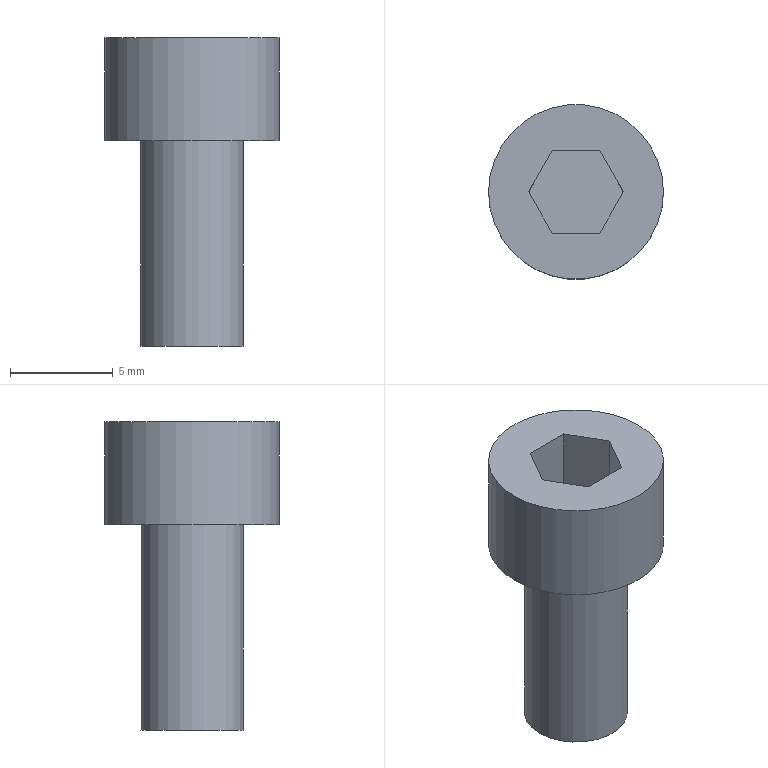Part | STEP file | lll_id514_x_t | 1 solid | 12 faces | box 8.5 x 8.5 x 15 mm | volume 434.348 mm3 | plane 10 | cylinder 2 | commonest cylinder face diameters 5 x1 8.5 x1
STEP:
#1=CARTESIAN_POINT('',(-8.75,0.,127.));
#2=VERTEX_POINT('',#1);
#3=CARTESIAN_POINT('',(-13.,0.,127.));
#4=DIRECTION('',(0.,0.,1.));
#5=DIRECTION('',(1.,0.,0.));
#6=AXIS2_PLACEMENT_3D('',#3,#4,#5);
#7=CIRCLE('',#6,4.25);
#8=EDGE_CURVE('',#2,#2,#7,.T.);
#9=ORIENTED_EDGE('',*,*,#8,.T.);
#10=EDGE_LOOP('',(#9));
#11=FACE_BOUND('',#10,.T.);
#12=CARTESIAN_POINT('',(-14.155,2.,127.));
#13=VERTEX_POINT('',#12);
#14=CARTESIAN_POINT('',(-11.845,2.,127.));
#15=VERTEX_POINT('',#14);
#16=CARTESIAN_POINT('',(-14.155,2.,127.));
#17=DIRECTION('',(1.,0.,0.));
#18=VECTOR('',#17,1.);
#19=LINE('',#16,#18);
#20=EDGE_CURVE('',#13,#15,#19,.T.);
#21=ORIENTED_EDGE('',*,*,#20,.T.);
#22=CARTESIAN_POINT('',(-10.691,0.,127.));
#23=VERTEX_POINT('',#22);
#24=CARTESIAN_POINT('',(-11.845,2.,127.));
#25=DIRECTION('',(0.5,-0.866,0.));
#26=VECTOR('',#25,1.);
#27=LINE('',#24,#26);
#28=EDGE_CURVE('',#15,#23,#27,.T.);
#29=ORIENTED_EDGE('',*,*,#28,.T.);
#30=CARTESIAN_POINT('',(-11.845,-2.,127.));
#31=VERTEX_POINT('',#30);
#32=CARTESIAN_POINT('',(-10.691,0.,127.));
#33=DIRECTION('',(-0.5,-0.866,0.));
#34=VECTOR('',#33,1.);
#35=LINE('',#32,#34);
#36=EDGE_CURVE('',#23,#31,#35,.T.);
#37=ORIENTED_EDGE('',*,*,#36,.T.);
#38=CARTESIAN_POINT('',(-14.155,-2.,127.));
#39=VERTEX_POINT('',#38);
#40=CARTESIAN_POINT('',(-11.845,-2.,127.));
#41=DIRECTION('',(-1.,0.,0.));
#42=VECTOR('',#41,1.);
#43=LINE('',#40,#42);
#44=EDGE_CURVE('',#31,#39,#43,.T.);
#45=ORIENTED_EDGE('',*,*,#44,.T.);
#46=CARTESIAN_POINT('',(-15.309,0.,127.));
#47=VERTEX_POINT('',#46);
#48=CARTESIAN_POINT('',(-14.155,-2.,127.));
#49=DIRECTION('',(-0.5,0.866,0.));
#50=VECTOR('',#49,1.);
#51=LINE('',#48,#50);
#52=EDGE_CURVE('',#39,#47,#51,.T.);
#53=ORIENTED_EDGE('',*,*,#52,.T.);
#54=CARTESIAN_POINT('',(-15.309,0.,127.));
#55=DIRECTION('',(0.5,0.866,0.));
#56=VECTOR('',#55,1.);
#57=LINE('',#54,#56);
#58=EDGE_CURVE('',#47,#13,#57,.T.);
#59=ORIENTED_EDGE('',*,*,#58,.T.);
#60=EDGE_LOOP('',(#21,#29,#37,#45,#53,#59));
#61=FACE_BOUND('',#60,.T.);
#62=CARTESIAN_POINT('',(-8.75,0.,127.));
#63=DIRECTION('',(0.,0.,-1.));
#64=DIRECTION('',(-1.,0.,0.));
#65=AXIS2_PLACEMENT_3D('',#62,#63,#64);
#66=PLANE('',#65);
#67=ADVANCED_FACE('',(#11,#61),#66,.F.);
#68=ORIENTED_EDGE('',*,*,#8,.F.);
#69=EDGE_LOOP('',(#68));
#70=FACE_BOUND('',#69,.T.);
#71=CARTESIAN_POINT('',(-8.75,0.,122.));
#72=VERTEX_POINT('',#71);
#73=CARTESIAN_POINT('',(-13.,0.,122.));
#74=DIRECTION('',(0.,0.,1.));
#75=DIRECTION('',(1.,0.,0.));
#76=AXIS2_PLACEMENT_3D('',#73,#74,#75);
#77=CIRCLE('',#76,4.25);
#78=EDGE_CURVE('',#72,#72,#77,.T.);
#79=ORIENTED_EDGE('',*,*,#78,.T.);
#80=EDGE_LOOP('',(#79));
#81=FACE_BOUND('',#80,.T.);
#82=CARTESIAN_POINT('',(-13.,0.,120.6));
#83=DIRECTION('',(0.,0.,1.));
#84=DIRECTION('',(1.,0.,0.));
#85=AXIS2_PLACEMENT_3D('',#82,#83,#84);
#86=CYLINDRICAL_SURFACE('',#85,4.25);
#87=ADVANCED_FACE('',(#70,#81),#86,.T.);
#88=ORIENTED_EDGE('',*,*,#78,.F.);
#89=EDGE_LOOP('',(#88));
#90=FACE_BOUND('',#89,.T.);
#91=CARTESIAN_POINT('',(-10.5,0.,122.));
#92=VERTEX_POINT('',#91);
#93=CARTESIAN_POINT('',(-13.,0.,122.));
#94=DIRECTION('',(0.,0.,1.));
#95=DIRECTION('',(1.,0.,0.));
#96=AXIS2_PLACEMENT_3D('',#93,#94,#95);
#97=CIRCLE('',#96,2.5);
#98=EDGE_CURVE('',#92,#92,#97,.T.);
#99=ORIENTED_EDGE('',*,*,#98,.T.);
#100=EDGE_LOOP('',(#99));
#101=FACE_BOUND('',#100,.T.);
#102=CARTESIAN_POINT('',(-10.5,0.,122.));
#103=DIRECTION('',(0.,0.,1.));
#104=DIRECTION('',(1.,0.,0.));
#105=AXIS2_PLACEMENT_3D('',#102,#103,#104);
#106=PLANE('',#105);
#107=ADVANCED_FACE('',(#90,#101),#106,.F.);
#108=ORIENTED_EDGE('',*,*,#98,.F.);
#109=EDGE_LOOP('',(#108));
#110=FACE_BOUND('',#109,.T.);
#111=CARTESIAN_POINT('',(-10.5,0.,112.));
#112=VERTEX_POINT('',#111);
#113=CARTESIAN_POINT('',(-13.,0.,112.));
#114=DIRECTION('',(0.,0.,1.));
#115=DIRECTION('',(1.,0.,0.));
#116=AXIS2_PLACEMENT_3D('',#113,#114,#115);
#117=CIRCLE('',#116,2.5);
#118=EDGE_CURVE('',#112,#112,#117,.T.);
#119=ORIENTED_EDGE('',*,*,#118,.T.);
#120=EDGE_LOOP('',(#119));
#121=FACE_BOUND('',#120,.T.);
#122=CARTESIAN_POINT('',(-13.,0.,120.6));
#123=DIRECTION('',(0.,0.,1.));
#124=DIRECTION('',(1.,0.,0.));
#125=AXIS2_PLACEMENT_3D('',#122,#123,#124);
#126=CYLINDRICAL_SURFACE('',#125,2.5);
#127=ADVANCED_FACE('',(#110,#121),#126,.T.);
#128=ORIENTED_EDGE('',*,*,#118,.F.);
#129=EDGE_LOOP('',(#128));
#130=FACE_OUTER_BOUND('',#129,.T.);
#131=CARTESIAN_POINT('',(-13.,0.,112.));
#132=DIRECTION('',(0.,0.,1.));
#133=DIRECTION('',(1.,0.,0.));
#134=AXIS2_PLACEMENT_3D('',#131,#132,#133);
#135=PLANE('',#134);
#136=ADVANCED_FACE('',(#130),#135,.F.);
#137=ORIENTED_EDGE('',*,*,#20,.F.);
#138=CARTESIAN_POINT('',(-14.155,2.,123.7));
#139=VERTEX_POINT('',#138);
#140=CARTESIAN_POINT('',(-14.155,2.,123.7));
#141=DIRECTION('',(0.,0.,-1.));
#142=VECTOR('',#141,1.);
#143=LINE('',#140,#142);
#144=EDGE_CURVE('',#13,#139,#143,.T.);
#145=ORIENTED_EDGE('',*,*,#144,.T.);
#146=CARTESIAN_POINT('',(-11.845,2.,123.7));
#147=VERTEX_POINT('',#146);
#148=CARTESIAN_POINT('',(-14.155,2.,123.7));
#149=DIRECTION('',(-1.,0.,0.));
#150=VECTOR('',#149,1.);
#151=LINE('',#148,#150);
#152=EDGE_CURVE('',#147,#139,#151,.T.);
#153=ORIENTED_EDGE('',*,*,#152,.F.);
#154=CARTESIAN_POINT('',(-11.845,2.,123.7));
#155=DIRECTION('',(0.,0.,-1.));
#156=VECTOR('',#155,1.);
#157=LINE('',#154,#156);
#158=EDGE_CURVE('',#15,#147,#157,.T.);
#159=ORIENTED_EDGE('',*,*,#158,.F.);
#160=EDGE_LOOP('',(#137,#145,#153,#159));
#161=FACE_OUTER_BOUND('',#160,.T.);
#162=CARTESIAN_POINT('',(-14.155,2.,123.7));
#163=DIRECTION('',(0.,-1.,0.));
#164=DIRECTION('',(1.,0.,0.));
#165=AXIS2_PLACEMENT_3D('',#162,#163,#164);
#166=PLANE('',#165);
#167=ADVANCED_FACE('',(#161),#166,.T.);
#168=ORIENTED_EDGE('',*,*,#28,.F.);
#169=ORIENTED_EDGE('',*,*,#158,.T.);
#170=CARTESIAN_POINT('',(-10.691,0.,123.7));
#171=VERTEX_POINT('',#170);
#172=CARTESIAN_POINT('',(-11.845,2.,123.7));
#173=DIRECTION('',(-0.5,0.866,0.));
#174=VECTOR('',#173,1.);
#175=LINE('',#172,#174);
#176=EDGE_CURVE('',#171,#147,#175,.T.);
#177=ORIENTED_EDGE('',*,*,#176,.F.);
#178=CARTESIAN_POINT('',(-10.691,0.,123.7));
#179=DIRECTION('',(0.,0.,-1.));
#180=VECTOR('',#179,1.);
#181=LINE('',#178,#180);
#182=EDGE_CURVE('',#23,#171,#181,.T.);
#183=ORIENTED_EDGE('',*,*,#182,.F.);
#184=EDGE_LOOP('',(#168,#169,#177,#183));
#185=FACE_OUTER_BOUND('',#184,.T.);
#186=CARTESIAN_POINT('',(-11.845,2.,123.7));
#187=DIRECTION('',(-0.866,-0.5,0.));
#188=DIRECTION('',(0.5,-0.866,0.));
#189=AXIS2_PLACEMENT_3D('',#186,#187,#188);
#190=PLANE('',#189);
#191=ADVANCED_FACE('',(#185),#190,.T.);
#192=ORIENTED_EDGE('',*,*,#36,.F.);
#193=ORIENTED_EDGE('',*,*,#182,.T.);
#194=CARTESIAN_POINT('',(-11.845,-2.,123.7));
#195=VERTEX_POINT('',#194);
#196=CARTESIAN_POINT('',(-10.691,0.,123.7));
#197=DIRECTION('',(0.5,0.866,0.));
#198=VECTOR('',#197,1.);
#199=LINE('',#196,#198);
#200=EDGE_CURVE('',#195,#171,#199,.T.);
#201=ORIENTED_EDGE('',*,*,#200,.F.);
#202=CARTESIAN_POINT('',(-11.845,-2.,123.7));
#203=DIRECTION('',(0.,0.,-1.));
#204=VECTOR('',#203,1.);
#205=LINE('',#202,#204);
#206=EDGE_CURVE('',#31,#195,#205,.T.);
#207=ORIENTED_EDGE('',*,*,#206,.F.);
#208=EDGE_LOOP('',(#192,#193,#201,#207));
#209=FACE_OUTER_BOUND('',#208,.T.);
#210=CARTESIAN_POINT('',(-10.691,0.,123.7));
#211=DIRECTION('',(-0.866,0.5,0.));
#212=DIRECTION('',(-0.5,-0.866,0.));
#213=AXIS2_PLACEMENT_3D('',#210,#211,#212);
#214=PLANE('',#213);
#215=ADVANCED_FACE('',(#209),#214,.T.);
#216=ORIENTED_EDGE('',*,*,#44,.F.);
#217=ORIENTED_EDGE('',*,*,#206,.T.);
#218=CARTESIAN_POINT('',(-14.155,-2.,123.7));
#219=VERTEX_POINT('',#218);
#220=CARTESIAN_POINT('',(-11.845,-2.,123.7));
#221=DIRECTION('',(1.,0.,0.));
#222=VECTOR('',#221,1.);
#223=LINE('',#220,#222);
#224=EDGE_CURVE('',#219,#195,#223,.T.);
#225=ORIENTED_EDGE('',*,*,#224,.F.);
#226=CARTESIAN_POINT('',(-14.155,-2.,123.7));
#227=DIRECTION('',(0.,0.,-1.));
#228=VECTOR('',#227,1.);
#229=LINE('',#226,#228);
#230=EDGE_CURVE('',#39,#219,#229,.T.);
#231=ORIENTED_EDGE('',*,*,#230,.F.);
#232=EDGE_LOOP('',(#216,#217,#225,#231));
#233=FACE_OUTER_BOUND('',#232,.T.);
#234=CARTESIAN_POINT('',(-11.845,-2.,123.7));
#235=DIRECTION('',(0.,1.,0.));
#236=DIRECTION('',(-1.,0.,0.));
#237=AXIS2_PLACEMENT_3D('',#234,#235,#236);
#238=PLANE('',#237);
#239=ADVANCED_FACE('',(#233),#238,.T.);
#240=ORIENTED_EDGE('',*,*,#52,.F.);
#241=ORIENTED_EDGE('',*,*,#230,.T.);
#242=CARTESIAN_POINT('',(-15.309,0.,123.7));
#243=VERTEX_POINT('',#242);
#244=CARTESIAN_POINT('',(-14.155,-2.,123.7));
#245=DIRECTION('',(0.5,-0.866,0.));
#246=VECTOR('',#245,1.);
#247=LINE('',#244,#246);
#248=EDGE_CURVE('',#243,#219,#247,.T.);
#249=ORIENTED_EDGE('',*,*,#248,.F.);
#250=CARTESIAN_POINT('',(-15.309,0.,123.7));
#251=DIRECTION('',(0.,0.,-1.));
#252=VECTOR('',#251,1.);
#253=LINE('',#250,#252);
#254=EDGE_CURVE('',#47,#243,#253,.T.);
#255=ORIENTED_EDGE('',*,*,#254,.F.);
#256=EDGE_LOOP('',(#240,#241,#249,#255));
#257=FACE_OUTER_BOUND('',#256,.T.);
#258=CARTESIAN_POINT('',(-14.155,-2.,123.7));
#259=DIRECTION('',(0.866,0.5,0.));
#260=DIRECTION('',(-0.5,0.866,0.));
#261=AXIS2_PLACEMENT_3D('',#258,#259,#260);
#262=PLANE('',#261);
#263=ADVANCED_FACE('',(#257),#262,.T.);
#264=ORIENTED_EDGE('',*,*,#58,.F.);
#265=ORIENTED_EDGE('',*,*,#254,.T.);
#266=CARTESIAN_POINT('',(-15.309,0.,123.7));
#267=DIRECTION('',(-0.5,-0.866,0.));
#268=VECTOR('',#267,1.);
#269=LINE('',#266,#268);
#270=EDGE_CURVE('',#139,#243,#269,.T.);
#271=ORIENTED_EDGE('',*,*,#270,.F.);
#272=ORIENTED_EDGE('',*,*,#144,.F.);
#273=EDGE_LOOP('',(#264,#265,#271,#272));
#274=FACE_OUTER_BOUND('',#273,.T.);
#275=CARTESIAN_POINT('',(-15.309,0.,123.7));
#276=DIRECTION('',(0.866,-0.5,0.));
#277=DIRECTION('',(0.5,0.866,0.));
#278=AXIS2_PLACEMENT_3D('',#275,#276,#277);
#279=PLANE('',#278);
#280=ADVANCED_FACE('',(#274),#279,.T.);
#281=ORIENTED_EDGE('',*,*,#152,.T.);
#282=ORIENTED_EDGE('',*,*,#270,.T.);
#283=ORIENTED_EDGE('',*,*,#248,.T.);
#284=ORIENTED_EDGE('',*,*,#224,.T.);
#285=ORIENTED_EDGE('',*,*,#200,.T.);
#286=ORIENTED_EDGE('',*,*,#176,.T.);
#287=EDGE_LOOP('',(#281,#282,#283,#284,#285,#286));
#288=FACE_OUTER_BOUND('',#287,.T.);
#289=CARTESIAN_POINT('',(-13.,0.,123.7));
#290=DIRECTION('',(0.,0.,-1.));
#291=DIRECTION('',(-1.,0.,0.));
#292=AXIS2_PLACEMENT_3D('',#289,#290,#291);
#293=PLANE('',#292);
#294=ADVANCED_FACE('',(#288),#293,.F.);
#295=CLOSED_SHELL('',(#67,#87,#107,#127,#136,#167,#191,#215,#239,#263,#280,#294));
#296=MANIFOLD_SOLID_BREP('',#295);
#297=(LENGTH_UNIT()NAMED_UNIT(*)SI_UNIT(.MILLI.,.METRE.));
#298=UNCERTAINTY_MEASURE_WITH_UNIT(LENGTH_MEASURE(0.00002),#297,'','');
#299=(NAMED_UNIT(*)PLANE_ANGLE_UNIT()SI_UNIT($,.RADIAN.));
#300=PLANE_ANGLE_MEASURE_WITH_UNIT(PLANE_ANGLE_MEASURE(0.01745),#299);
#301=DIMENSIONAL_EXPONENTS(0.,0.,0.,0.,0.,0.,0.);
#302=(CONVERSION_BASED_UNIT('DEGREE',#300)NAMED_UNIT(#301)PLANE_ANGLE_UNIT());
#303=(NAMED_UNIT(*)SI_UNIT($,.STERADIAN.)SOLID_ANGLE_UNIT());
#304=(GEOMETRIC_REPRESENTATION_CONTEXT(3)GLOBAL_UNCERTAINTY_ASSIGNED_CONTEXT((#298))GLOBAL_UNIT_ASSIGNED_CONTEXT((#297,#302,#303))REPRESENTATION_CONTEXT('',''));
#305=ADVANCED_BREP_SHAPE_REPRESENTATION('',(#296),#304);